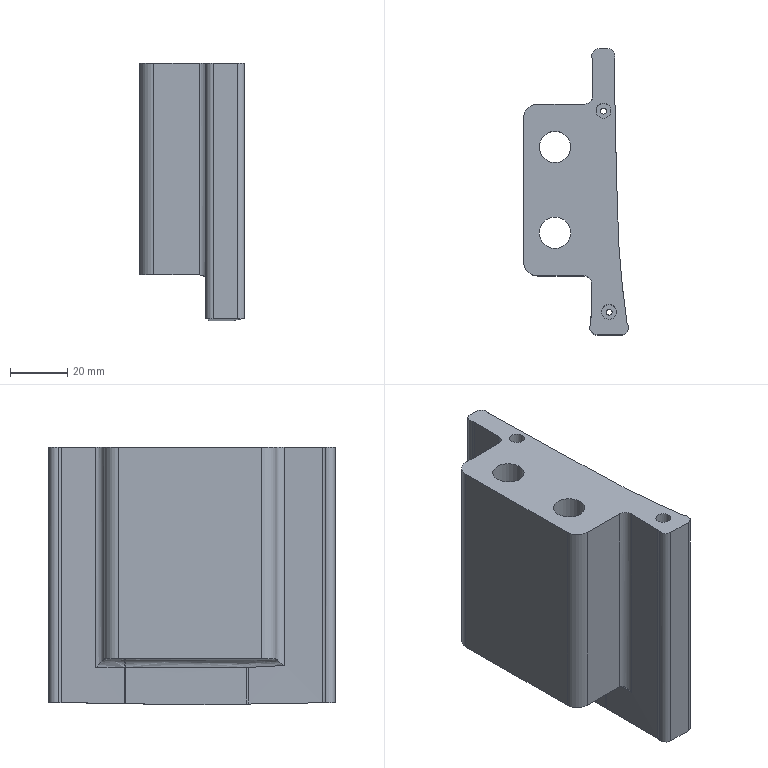Part | STEP file | gslz 2016.10.28-10_id3050_x_t | 1 solid | 45 faces | box 36.691 x 100 x 90 mm | volume 156614 mm3 | cylinder 21 | plane 17 | other 5 | spline 2 | commonest cylinder face diameters 5 x8 6 x3 2.1 x2 5.2 x2 10 x2 11 x2